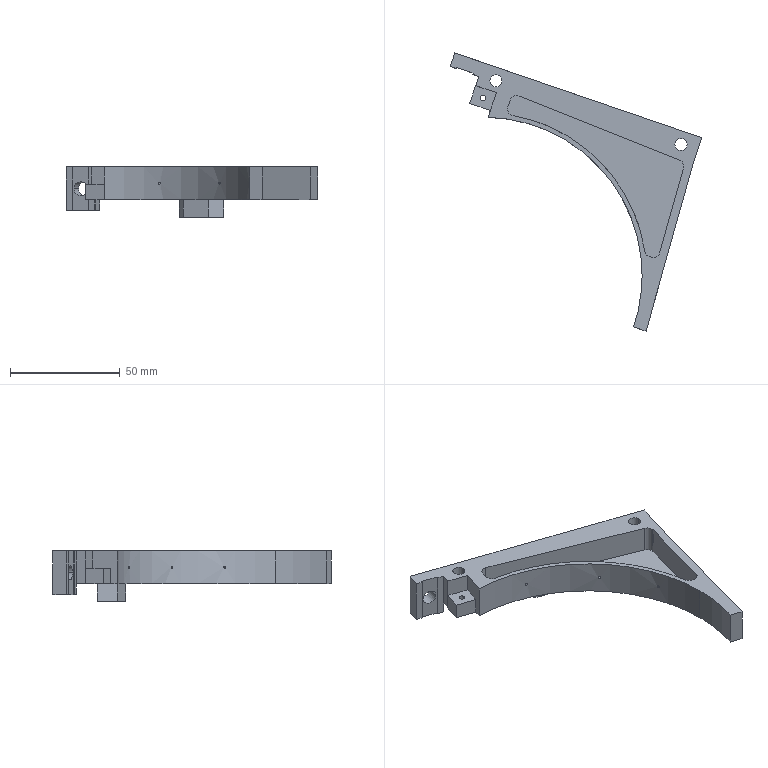Part | SolidWorks | features Cut 5, ICE 5, RevCut 3, HoleWzd 2, Extrusion 1 | 1 solid | 55 faces | box 114.513 x 126.581 x 23 mm | volume 34944 mm3 | plane 32 | cylinder 23 | commonest cylinder face diameters 1 x6 6 x6 5.5 x4 2.5 x2 6.5 x2 144 x2